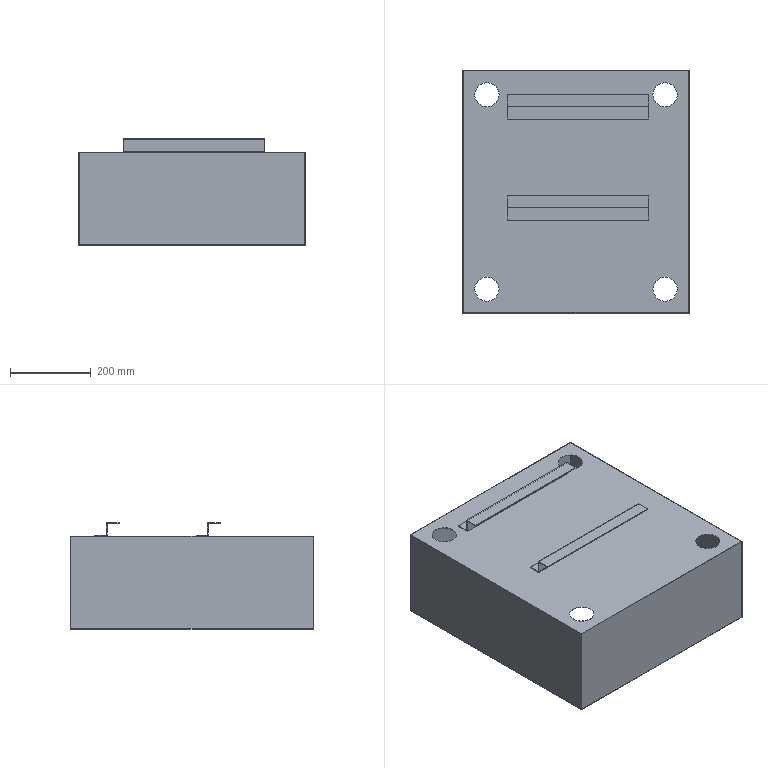Part | SolidWorks | features BaseBody 1 | 1 solid | 47 faces | box 560 x 600 x 263 mm | volume 1044894 mm3 | plane 39 | cylinder 8 | commonest cylinder face diameters 60 x8
STEP:
#1=CARTESIAN_POINT('',(530.,540.,230.));
#2=VERTEX_POINT('',#1);
#3=CARTESIAN_POINT('',(470.,540.,230.));
#4=VERTEX_POINT('',#3);
#5=CARTESIAN_POINT('',(500.,540.,230.));
#6=DIRECTION('',(0.,0.,-1.));
#7=DIRECTION('',(-1.,0.,0.));
#8=AXIS2_PLACEMENT_3D('',#5,#6,#7);
#9=CIRCLE('',#8,30.);
#10=EDGE_CURVE('',#2,#4,#9,.T.);
#11=ORIENTED_EDGE('',*,*,#10,.F.);
#12=CARTESIAN_POINT('',(530.,540.,229.));
#13=VERTEX_POINT('',#12);
#14=CARTESIAN_POINT('',(530.,540.,263.));
#15=DIRECTION('',(0.,0.,-1.));
#16=VECTOR('',#15,1000.);
#17=LINE('',#14,#16);
#18=EDGE_CURVE('',#2,#13,#17,.T.);
#19=ORIENTED_EDGE('',*,*,#18,.T.);
#20=CARTESIAN_POINT('',(470.,540.,229.));
#21=VERTEX_POINT('',#20);
#22=CARTESIAN_POINT('',(500.,540.,229.));
#23=DIRECTION('',(0.,0.,1.));
#24=DIRECTION('',(-1.,0.,0.));
#25=AXIS2_PLACEMENT_3D('',#22,#23,#24);
#26=CIRCLE('',#25,30.);
#27=EDGE_CURVE('',#21,#13,#26,.T.);
#28=ORIENTED_EDGE('',*,*,#27,.F.);
#29=CARTESIAN_POINT('',(470.,540.,263.));
#30=DIRECTION('',(0.,0.,-1.));
#31=VECTOR('',#30,1000.);
#32=LINE('',#29,#31);
#33=EDGE_CURVE('',#4,#21,#32,.T.);
#34=ORIENTED_EDGE('',*,*,#33,.F.);
#35=EDGE_LOOP('',(#11,#19,#28,#34));
#36=FACE_OUTER_BOUND('',#35,.T.);
#37=CARTESIAN_POINT('',(500.,540.,263.));
#38=DIRECTION('',(0.,0.,-1.));
#39=DIRECTION('',(-1.,0.,0.));
#40=AXIS2_PLACEMENT_3D('',#37,#38,#39);
#41=CYLINDRICAL_SURFACE('',#40,30.);
#42=ADVANCED_FACE('',(#36),#41,.F.);
#43=CARTESIAN_POINT('',(90.,540.,230.));
#44=VERTEX_POINT('',#43);
#45=CARTESIAN_POINT('',(30.,540.,230.));
#46=VERTEX_POINT('',#45);
#47=CARTESIAN_POINT('',(60.,540.,230.));
#48=DIRECTION('',(0.,0.,-1.));
#49=DIRECTION('',(-1.,0.,0.));
#50=AXIS2_PLACEMENT_3D('',#47,#48,#49);
#51=CIRCLE('',#50,30.);
#52=EDGE_CURVE('',#44,#46,#51,.T.);
#53=ORIENTED_EDGE('',*,*,#52,.F.);
#54=CARTESIAN_POINT('',(90.,540.,229.));
#55=VERTEX_POINT('',#54);
#56=CARTESIAN_POINT('',(90.,540.,263.));
#57=DIRECTION('',(0.,0.,-1.));
#58=VECTOR('',#57,1000.);
#59=LINE('',#56,#58);
#60=EDGE_CURVE('',#44,#55,#59,.T.);
#61=ORIENTED_EDGE('',*,*,#60,.T.);
#62=CARTESIAN_POINT('',(30.,540.,229.));
#63=VERTEX_POINT('',#62);
#64=CARTESIAN_POINT('',(60.,540.,229.));
#65=DIRECTION('',(0.,0.,1.));
#66=DIRECTION('',(-1.,0.,0.));
#67=AXIS2_PLACEMENT_3D('',#64,#65,#66);
#68=CIRCLE('',#67,30.);
#69=EDGE_CURVE('',#63,#55,#68,.T.);
#70=ORIENTED_EDGE('',*,*,#69,.F.);
#71=CARTESIAN_POINT('',(30.,540.,263.));
#72=DIRECTION('',(0.,0.,-1.));
#73=VECTOR('',#72,1000.);
#74=LINE('',#71,#73);
#75=EDGE_CURVE('',#46,#63,#74,.T.);
#76=ORIENTED_EDGE('',*,*,#75,.F.);
#77=EDGE_LOOP('',(#53,#61,#70,#76));
#78=FACE_OUTER_BOUND('',#77,.T.);
#79=CARTESIAN_POINT('',(60.,540.,263.));
#80=DIRECTION('',(0.,0.,-1.));
#81=DIRECTION('',(-1.,0.,0.));
#82=AXIS2_PLACEMENT_3D('',#79,#80,#81);
#83=CYLINDRICAL_SURFACE('',#82,30.);
#84=ADVANCED_FACE('',(#78),#83,.F.);
#85=CARTESIAN_POINT('',(90.,60.,230.));
#86=VERTEX_POINT('',#85);
#87=CARTESIAN_POINT('',(30.,60.,230.));
#88=VERTEX_POINT('',#87);
#89=CARTESIAN_POINT('',(60.,60.,230.));
#90=DIRECTION('',(0.,0.,-1.));
#91=DIRECTION('',(-1.,0.,0.));
#92=AXIS2_PLACEMENT_3D('',#89,#90,#91);
#93=CIRCLE('',#92,30.);
#94=EDGE_CURVE('',#86,#88,#93,.T.);
#95=ORIENTED_EDGE('',*,*,#94,.F.);
#96=CARTESIAN_POINT('',(90.,60.,229.));
#97=VERTEX_POINT('',#96);
#98=CARTESIAN_POINT('',(90.,60.,263.));
#99=DIRECTION('',(0.,0.,-1.));
#100=VECTOR('',#99,1000.);
#101=LINE('',#98,#100);
#102=EDGE_CURVE('',#86,#97,#101,.T.);
#103=ORIENTED_EDGE('',*,*,#102,.T.);
#104=CARTESIAN_POINT('',(30.,60.,229.));
#105=VERTEX_POINT('',#104);
#106=CARTESIAN_POINT('',(60.,60.,229.));
#107=DIRECTION('',(0.,0.,1.));
#108=DIRECTION('',(-1.,0.,0.));
#109=AXIS2_PLACEMENT_3D('',#106,#107,#108);
#110=CIRCLE('',#109,30.);
#111=EDGE_CURVE('',#105,#97,#110,.T.);
#112=ORIENTED_EDGE('',*,*,#111,.F.);
#113=CARTESIAN_POINT('',(30.,60.,263.));
#114=DIRECTION('',(0.,0.,-1.));
#115=VECTOR('',#114,1000.);
#116=LINE('',#113,#115);
#117=EDGE_CURVE('',#88,#105,#116,.T.);
#118=ORIENTED_EDGE('',*,*,#117,.F.);
#119=EDGE_LOOP('',(#95,#103,#112,#118));
#120=FACE_OUTER_BOUND('',#119,.T.);
#121=CARTESIAN_POINT('',(60.,60.,263.));
#122=DIRECTION('',(0.,0.,-1.));
#123=DIRECTION('',(-1.,0.,0.));
#124=AXIS2_PLACEMENT_3D('',#121,#122,#123);
#125=CYLINDRICAL_SURFACE('',#124,30.);
#126=ADVANCED_FACE('',(#120),#125,.F.);
#127=CARTESIAN_POINT('',(530.,60.,230.));
#128=VERTEX_POINT('',#127);
#129=CARTESIAN_POINT('',(470.,60.,230.));
#130=VERTEX_POINT('',#129);
#131=CARTESIAN_POINT('',(500.,60.,230.));
#132=DIRECTION('',(0.,0.,-1.));
#133=DIRECTION('',(-1.,0.,0.));
#134=AXIS2_PLACEMENT_3D('',#131,#132,#133);
#135=CIRCLE('',#134,30.);
#136=EDGE_CURVE('',#128,#130,#135,.T.);
#137=ORIENTED_EDGE('',*,*,#136,.F.);
#138=CARTESIAN_POINT('',(530.,60.,229.));
#139=VERTEX_POINT('',#138);
#140=CARTESIAN_POINT('',(530.,60.,263.));
#141=DIRECTION('',(0.,0.,-1.));
#142=VECTOR('',#141,1000.);
#143=LINE('',#140,#142);
#144=EDGE_CURVE('',#128,#139,#143,.T.);
#145=ORIENTED_EDGE('',*,*,#144,.T.);
#146=CARTESIAN_POINT('',(470.,60.,229.));
#147=VERTEX_POINT('',#146);
#148=CARTESIAN_POINT('',(500.,60.,229.));
#149=DIRECTION('',(0.,0.,1.));
#150=DIRECTION('',(-1.,0.,0.));
#151=AXIS2_PLACEMENT_3D('',#148,#149,#150);
#152=CIRCLE('',#151,30.);
#153=EDGE_CURVE('',#147,#139,#152,.T.);
#154=ORIENTED_EDGE('',*,*,#153,.F.);
#155=CARTESIAN_POINT('',(470.,60.,263.));
#156=DIRECTION('',(0.,0.,-1.));
#157=VECTOR('',#156,1000.);
#158=LINE('',#155,#157);
#159=EDGE_CURVE('',#130,#147,#158,.T.);
#160=ORIENTED_EDGE('',*,*,#159,.F.);
#161=EDGE_LOOP('',(#137,#145,#154,#160));
#162=FACE_OUTER_BOUND('',#161,.T.);
#163=CARTESIAN_POINT('',(500.,60.,263.));
#164=DIRECTION('',(0.,0.,-1.));
#165=DIRECTION('',(-1.,0.,0.));
#166=AXIS2_PLACEMENT_3D('',#163,#164,#165);
#167=CYLINDRICAL_SURFACE('',#166,30.);
#168=ADVANCED_FACE('',(#162),#167,.F.);
#169=CARTESIAN_POINT('',(559.,599.,229.));
#170=VERTEX_POINT('',#169);
#171=CARTESIAN_POINT('',(559.,1.,229.));
#172=VERTEX_POINT('',#171);
#173=CARTESIAN_POINT('',(559.,0.,229.));
#174=DIRECTION('',(0.,-1.,0.));
#175=VECTOR('',#174,1000.);
#176=LINE('',#173,#175);
#177=EDGE_CURVE('',#170,#172,#176,.T.);
#178=ORIENTED_EDGE('',*,*,#177,.T.);
#179=CARTESIAN_POINT('',(1.,1.,229.));
#180=VERTEX_POINT('',#179);
#181=CARTESIAN_POINT('',(0.,1.,229.));
#182=DIRECTION('',(-1.,0.,0.));
#183=VECTOR('',#182,1000.);
#184=LINE('',#181,#183);
#185=EDGE_CURVE('',#172,#180,#184,.T.);
#186=ORIENTED_EDGE('',*,*,#185,.T.);
#187=CARTESIAN_POINT('',(1.,599.,229.));
#188=VERTEX_POINT('',#187);
#189=CARTESIAN_POINT('',(1.,0.,229.));
#190=DIRECTION('',(0.,1.,0.));
#191=VECTOR('',#190,1000.);
#192=LINE('',#189,#191);
#193=EDGE_CURVE('',#180,#188,#192,.T.);
#194=ORIENTED_EDGE('',*,*,#193,.T.);
#195=CARTESIAN_POINT('',(0.,599.,229.));
#196=DIRECTION('',(1.,0.,0.));
#197=VECTOR('',#196,1000.);
#198=LINE('',#195,#197);
#199=EDGE_CURVE('',#188,#170,#198,.T.);
#200=ORIENTED_EDGE('',*,*,#199,.T.);
#201=EDGE_LOOP('',(#178,#186,#194,#200));
#202=FACE_OUTER_BOUND('',#201,.T.);
#203=ORIENTED_EDGE('',*,*,#27,.T.);
#204=CARTESIAN_POINT('',(500.,540.,229.));
#205=DIRECTION('',(0.,0.,1.));
#206=DIRECTION('',(-1.,0.,0.));
#207=AXIS2_PLACEMENT_3D('',#204,#205,#206);
#208=CIRCLE('',#207,30.);
#209=EDGE_CURVE('',#13,#21,#208,.T.);
#210=ORIENTED_EDGE('',*,*,#209,.T.);
#211=EDGE_LOOP('',(#203,#210));
#212=FACE_BOUND('',#211,.T.);
#213=ORIENTED_EDGE('',*,*,#69,.T.);
#214=CARTESIAN_POINT('',(60.,540.,229.));
#215=DIRECTION('',(0.,0.,1.));
#216=DIRECTION('',(-1.,0.,0.));
#217=AXIS2_PLACEMENT_3D('',#214,#215,#216);
#218=CIRCLE('',#217,30.);
#219=EDGE_CURVE('',#55,#63,#218,.T.);
#220=ORIENTED_EDGE('',*,*,#219,.T.);
#221=EDGE_LOOP('',(#213,#220));
#222=FACE_BOUND('',#221,.T.);
#223=ORIENTED_EDGE('',*,*,#111,.T.);
#224=CARTESIAN_POINT('',(60.,60.,229.));
#225=DIRECTION('',(0.,0.,1.));
#226=DIRECTION('',(-1.,0.,0.));
#227=AXIS2_PLACEMENT_3D('',#224,#225,#226);
#228=CIRCLE('',#227,30.);
#229=EDGE_CURVE('',#97,#105,#228,.T.);
#230=ORIENTED_EDGE('',*,*,#229,.T.);
#231=EDGE_LOOP('',(#223,#230));
#232=FACE_BOUND('',#231,.T.);
#233=ORIENTED_EDGE('',*,*,#153,.T.);
#234=CARTESIAN_POINT('',(500.,60.,229.));
#235=DIRECTION('',(0.,0.,1.));
#236=DIRECTION('',(-1.,0.,0.));
#237=AXIS2_PLACEMENT_3D('',#234,#235,#236);
#238=CIRCLE('',#237,30.);
#239=EDGE_CURVE('',#139,#147,#238,.T.);
#240=ORIENTED_EDGE('',*,*,#239,.T.);
#241=EDGE_LOOP('',(#233,#240));
#242=FACE_BOUND('',#241,.T.);
#243=CARTESIAN_POINT('',(0.,0.,229.));
#244=DIRECTION('',(0.,0.,-1.));
#245=DIRECTION('',(-1.,0.,0.));
#246=AXIS2_PLACEMENT_3D('',#243,#244,#245);
#247=PLANE('',#246);
#248=ADVANCED_FACE('',(#202,#212,#222,#232,#242),#247,.T.);
#249=ORIENTED_EDGE('',*,*,#185,.F.);
#250=CARTESIAN_POINT('',(559.,1.,1.));
#251=VERTEX_POINT('',#250);
#252=CARTESIAN_POINT('',(559.,1.,230.));
#253=DIRECTION('',(0.,0.,-1.));
#254=VECTOR('',#253,1000.);
#255=LINE('',#252,#254);
#256=EDGE_CURVE('',#172,#251,#255,.T.);
#257=ORIENTED_EDGE('',*,*,#256,.T.);
#258=CARTESIAN_POINT('',(1.,1.,1.));
#259=VERTEX_POINT('',#258);
#260=CARTESIAN_POINT('',(0.,1.,1.));
#261=DIRECTION('',(-1.,0.,0.));
#262=VECTOR('',#261,1000.);
#263=LINE('',#260,#262);
#264=EDGE_CURVE('',#251,#259,#263,.T.);
#265=ORIENTED_EDGE('',*,*,#264,.T.);
#266=CARTESIAN_POINT('',(1.,1.,230.));
#267=DIRECTION('',(0.,0.,1.));
#268=VECTOR('',#267,1000.);
#269=LINE('',#266,#268);
#270=EDGE_CURVE('',#259,#180,#269,.T.);
#271=ORIENTED_EDGE('',*,*,#270,.T.);
#272=EDGE_LOOP('',(#249,#257,#265,#271));
#273=FACE_OUTER_BOUND('',#272,.T.);
#274=CARTESIAN_POINT('',(0.,1.,230.));
#275=DIRECTION('',(0.,1.,0.));
#276=DIRECTION('',(0.,0.,1.));
#277=AXIS2_PLACEMENT_3D('',#274,#275,#276);
#278=PLANE('',#277);
#279=ADVANCED_FACE('',(#273),#278,.T.);
#280=ORIENTED_EDGE('',*,*,#177,.F.);
#281=CARTESIAN_POINT('',(559.,599.,1.));
#282=VERTEX_POINT('',#281);
#283=CARTESIAN_POINT('',(559.,599.,230.));
#284=DIRECTION('',(0.,0.,-1.));
#285=VECTOR('',#284,1000.);
#286=LINE('',#283,#285);
#287=EDGE_CURVE('',#170,#282,#286,.T.);
#288=ORIENTED_EDGE('',*,*,#287,.T.);
#289=CARTESIAN_POINT('',(559.,0.,1.));
#290=DIRECTION('',(0.,-1.,0.));
#291=VECTOR('',#290,1000.);
#292=LINE('',#289,#291);
#293=EDGE_CURVE('',#282,#251,#292,.T.);
#294=ORIENTED_EDGE('',*,*,#293,.T.);
#295=ORIENTED_EDGE('',*,*,#256,.F.);
#296=EDGE_LOOP('',(#280,#288,#294,#295));
#297=FACE_OUTER_BOUND('',#296,.T.);
#298=CARTESIAN_POINT('',(559.,0.,230.));
#299=DIRECTION('',(-1.,0.,0.));
#300=DIRECTION('',(0.,0.,1.));
#301=AXIS2_PLACEMENT_3D('',#298,#299,#300);
#302=PLANE('',#301);
#303=ADVANCED_FACE('',(#297),#302,.T.);
#304=ORIENTED_EDGE('',*,*,#199,.F.);
#305=CARTESIAN_POINT('',(1.,599.,1.));
#306=VERTEX_POINT('',#305);
#307=CARTESIAN_POINT('',(1.,599.,230.));
#308=DIRECTION('',(0.,0.,-1.));
#309=VECTOR('',#308,1000.);
#310=LINE('',#307,#309);
#311=EDGE_CURVE('',#188,#306,#310,.T.);
#312=ORIENTED_EDGE('',*,*,#311,.T.);
#313=CARTESIAN_POINT('',(0.,599.,1.));
#314=DIRECTION('',(1.,0.,0.));
#315=VECTOR('',#314,1000.);
#316=LINE('',#313,#315);
#317=EDGE_CURVE('',#306,#282,#316,.T.);
#318=ORIENTED_EDGE('',*,*,#317,.T.);
#319=ORIENTED_EDGE('',*,*,#287,.F.);
#320=EDGE_LOOP('',(#304,#312,#318,#319));
#321=FACE_OUTER_BOUND('',#320,.T.);
#322=CARTESIAN_POINT('',(0.,599.,230.));
#323=DIRECTION('',(0.,-1.,0.));
#324=DIRECTION('',(0.,0.,-1.));
#325=AXIS2_PLACEMENT_3D('',#322,#323,#324);
#326=PLANE('',#325);
#327=ADVANCED_FACE('',(#321),#326,.T.);
#328=ORIENTED_EDGE('',*,*,#193,.F.);
#329=ORIENTED_EDGE('',*,*,#270,.F.);
#330=CARTESIAN_POINT('',(1.,0.,1.));
#331=DIRECTION('',(0.,1.,0.));
#332=VECTOR('',#331,1000.);
#333=LINE('',#330,#332);
#334=EDGE_CURVE('',#259,#306,#333,.T.);
#335=ORIENTED_EDGE('',*,*,#334,.T.);
#336=ORIENTED_EDGE('',*,*,#311,.F.);
#337=EDGE_LOOP('',(#328,#329,#335,#336));
#338=FACE_OUTER_BOUND('',#337,.T.);
#339=CARTESIAN_POINT('',(1.,0.,230.));
#340=DIRECTION('',(1.,0.,0.));
#341=DIRECTION('',(0.,0.,-1.));
#342=AXIS2_PLACEMENT_3D('',#339,#340,#341);
#343=PLANE('',#342);
#344=ADVANCED_FACE('',(#338),#343,.T.);
#345=ORIENTED_EDGE('',*,*,#18,.F.);
#346=CARTESIAN_POINT('',(500.,540.,230.));
#347=DIRECTION('',(0.,0.,-1.));
#348=DIRECTION('',(-1.,0.,0.));
#349=AXIS2_PLACEMENT_3D('',#346,#347,#348);
#350=CIRCLE('',#349,30.);
#351=EDGE_CURVE('',#4,#2,#350,.T.);
#352=ORIENTED_EDGE('',*,*,#351,.F.);
#353=ORIENTED_EDGE('',*,*,#33,.T.);
#354=ORIENTED_EDGE('',*,*,#209,.F.);
#355=EDGE_LOOP('',(#345,#352,#353,#354));
#356=FACE_OUTER_BOUND('',#355,.T.);
#357=CARTESIAN_POINT('',(500.,540.,263.));
#358=DIRECTION('',(0.,0.,-1.));
#359=DIRECTION('',(-1.,0.,0.));
#360=AXIS2_PLACEMENT_3D('',#357,#358,#359);
#361=CYLINDRICAL_SURFACE('',#360,30.);
#362=ADVANCED_FACE('',(#356),#361,.F.);
#363=ORIENTED_EDGE('',*,*,#60,.F.);
#364=CARTESIAN_POINT('',(60.,540.,230.));
#365=DIRECTION('',(0.,0.,-1.));
#366=DIRECTION('',(-1.,0.,0.));
#367=AXIS2_PLACEMENT_3D('',#364,#365,#366);
#368=CIRCLE('',#367,30.);
#369=EDGE_CURVE('',#46,#44,#368,.T.);
#370=ORIENTED_EDGE('',*,*,#369,.F.);
#371=ORIENTED_EDGE('',*,*,#75,.T.);
#372=ORIENTED_EDGE('',*,*,#219,.F.);
#373=EDGE_LOOP('',(#363,#370,#371,#372));
#374=FACE_OUTER_BOUND('',#373,.T.);
#375=CARTESIAN_POINT('',(60.,540.,263.));
#376=DIRECTION('',(0.,0.,-1.));
#377=DIRECTION('',(-1.,0.,0.));
#378=AXIS2_PLACEMENT_3D('',#375,#376,#377);
#379=CYLINDRICAL_SURFACE('',#378,30.);
#380=ADVANCED_FACE('',(#374),#379,.F.);
#381=ORIENTED_EDGE('',*,*,#102,.F.);
#382=CARTESIAN_POINT('',(60.,60.,230.));
#383=DIRECTION('',(0.,0.,-1.));
#384=DIRECTION('',(-1.,0.,0.));
#385=AXIS2_PLACEMENT_3D('',#382,#383,#384);
#386=CIRCLE('',#385,30.);
#387=EDGE_CURVE('',#88,#86,#386,.T.);
#388=ORIENTED_EDGE('',*,*,#387,.F.);
#389=ORIENTED_EDGE('',*,*,#117,.T.);
#390=ORIENTED_EDGE('',*,*,#229,.F.);
#391=EDGE_LOOP('',(#381,#388,#389,#390));
#392=FACE_OUTER_BOUND('',#391,.T.);
#393=CARTESIAN_POINT('',(60.,60.,263.));
#394=DIRECTION('',(0.,0.,-1.));
#395=DIRECTION('',(-1.,0.,0.));
#396=AXIS2_PLACEMENT_3D('',#393,#394,#395);
#397=CYLINDRICAL_SURFACE('',#396,30.);
#398=ADVANCED_FACE('',(#392),#397,.F.);
#399=ORIENTED_EDGE('',*,*,#144,.F.);
#400=CARTESIAN_POINT('',(500.,60.,230.));
#401=DIRECTION('',(0.,0.,-1.));
#402=DIRECTION('',(-1.,0.,0.));
#403=AXIS2_PLACEMENT_3D('',#400,#401,#402);
#404=CIRCLE('',#403,30.);
#405=EDGE_CURVE('',#130,#128,#404,.T.);
#406=ORIENTED_EDGE('',*,*,#405,.F.);
#407=ORIENTED_EDGE('',*,*,#159,.T.);
#408=ORIENTED_EDGE('',*,*,#239,.F.);
#409=EDGE_LOOP('',(#399,#406,#407,#408));
#410=FACE_OUTER_BOUND('',#409,.T.);
#411=CARTESIAN_POINT('',(500.,60.,263.));
#412=DIRECTION('',(0.,0.,-1.));
#413=DIRECTION('',(-1.,0.,0.));
#414=AXIS2_PLACEMENT_3D('',#411,#412,#413);
#415=CYLINDRICAL_SURFACE('',#414,30.);
#416=ADVANCED_FACE('',(#410),#415,.F.);
#417=ORIENTED_EDGE('',*,*,#264,.F.);
#418=ORIENTED_EDGE('',*,*,#293,.F.);
#419=ORIENTED_EDGE('',*,*,#317,.F.);
#420=ORIENTED_EDGE('',*,*,#334,.F.);
#421=EDGE_LOOP('',(#417,#418,#419,#420));
#422=FACE_OUTER_BOUND('',#421,.T.);
#423=CARTESIAN_POINT('',(14.,14.,1.));
#424=VERTEX_POINT('',#423);
#425=CARTESIAN_POINT('',(546.,14.,1.));
#426=VERTEX_POINT('',#425);
#427=CARTESIAN_POINT('',(0.,14.,1.));
#428=DIRECTION('',(1.,0.,0.));
#429=VECTOR('',#428,1000.);
#430=LINE('',#427,#429);
#431=EDGE_CURVE('',#424,#426,#430,.T.);
#432=ORIENTED_EDGE('',*,*,#431,.F.);
#433=CARTESIAN_POINT('',(14.,586.,1.));
#434=VERTEX_POINT('',#433);
#435=CARTESIAN_POINT('',(14.,0.,1.));
#436=DIRECTION('',(0.,-1.,0.));
#437=VECTOR('',#436,1000.);
#438=LINE('',#435,#437);
#439=EDGE_CURVE('',#434,#424,#438,.T.);
#440=ORIENTED_EDGE('',*,*,#439,.F.);
#441=CARTESIAN_POINT('',(546.,586.,1.));
#442=VERTEX_POINT('',#441);
#443=CARTESIAN_POINT('',(0.,586.,1.));
#444=DIRECTION('',(-1.,0.,0.));
#445=VECTOR('',#444,1000.);
#446=LINE('',#443,#445);
#447=EDGE_CURVE('',#442,#434,#446,.T.);
#448=ORIENTED_EDGE('',*,*,#447,.F.);
#449=CARTESIAN_POINT('',(546.,0.,1.));
#450=DIRECTION('',(0.,1.,0.));
#451=VECTOR('',#450,1000.);
#452=LINE('',#449,#451);
#453=EDGE_CURVE('',#426,#442,#452,.T.);
#454=ORIENTED_EDGE('',*,*,#453,.F.);
#455=EDGE_LOOP('',(#432,#440,#448,#454));
#456=FACE_BOUND('',#455,.T.);
#457=CARTESIAN_POINT('',(0.,0.,1.));
#458=DIRECTION('',(0.,0.,-1.));
#459=DIRECTION('',(-1.,0.,0.));
#460=AXIS2_PLACEMENT_3D('',#457,#458,#459);
#461=PLANE('',#460);
#462=ADVANCED_FACE('',(#422,#456),#461,.F.);
#463=CARTESIAN_POINT('',(460.,290.,230.));
#464=VERTEX_POINT('',#463);
#465=CARTESIAN_POINT('',(110.,290.,230.));
#466=VERTEX_POINT('',#465);
#467=CARTESIAN_POINT('',(0.,290.,230.));
#468=DIRECTION('',(-1.,0.,0.));
#469=VECTOR('',#468,1000.);
#470=LINE('',#467,#469);
#471=EDGE_CURVE('',#464,#466,#470,.T.);
#472=ORIENTED_EDGE('',*,*,#471,.F.);
#473=CARTESIAN_POINT('',(460.,260.,230.));
#474=VERTEX_POINT('',#473);
#475=CARTESIAN_POINT('',(460.,0.,230.));
#476=DIRECTION('',(0.,1.,0.));
#477=VECTOR('',#476,1000.);
#478=LINE('',#475,#477);
#479=EDGE_CURVE('',#474,#464,#478,.T.);
#480=ORIENTED_EDGE('',*,*,#479,.F.);
#481=CARTESIAN_POINT('',(110.,260.,230.));
#482=VERTEX_POINT('',#481);
#483=CARTESIAN_POINT('',(0.,260.,230.));
#484=DIRECTION('',(1.,0.,0.));
#485=VECTOR('',#484,1000.);
#486=LINE('',#483,#485);
#487=EDGE_CURVE('',#482,#474,#486,.T.);
#488=ORIENTED_EDGE('',*,*,#487,.F.);
#489=CARTESIAN_POINT('',(110.,0.,230.));
#490=DIRECTION('',(0.,-1.,0.));
#491=VECTOR('',#490,1000.);
#492=LINE('',#489,#491);
#493=EDGE_CURVE('',#466,#482,#492,.T.);
#494=ORIENTED_EDGE('',*,*,#493,.F.);
#495=EDGE_LOOP('',(#472,#480,#488,#494));
#496=FACE_BOUND('',#495,.T.);
#497=CARTESIAN_POINT('',(560.,0.,230.));
#498=VERTEX_POINT('',#497);
#499=CARTESIAN_POINT('',(0.,0.,230.));
#500=VERTEX_POINT('',#499);
#501=CARTESIAN_POINT('',(0.,0.,230.));
#502=DIRECTION('',(-1.,0.,0.));
#503=VECTOR('',#502,1000.);
#504=LINE('',#501,#503);
#505=EDGE_CURVE('',#498,#500,#504,.T.);
#506=ORIENTED_EDGE('',*,*,#505,.F.);
#507=CARTESIAN_POINT('',(560.,600.,230.));
#508=VERTEX_POINT('',#507);
#509=CARTESIAN_POINT('',(560.,0.,230.));
#510=DIRECTION('',(0.,-1.,0.));
#511=VECTOR('',#510,1000.);
#512=LINE('',#509,#511);
#513=EDGE_CURVE('',#508,#498,#512,.T.);
#514=ORIENTED_EDGE('',*,*,#513,.F.);
#515=CARTESIAN_POINT('',(0.,600.,230.));
#516=VERTEX_POINT('',#515);
#517=CARTESIAN_POINT('',(0.,600.,230.));
#518=DIRECTION('',(1.,0.,0.));
#519=VECTOR('',#518,1000.);
#520=LINE('',#517,#519);
#521=EDGE_CURVE('',#516,#508,#520,.T.);
#522=ORIENTED_EDGE('',*,*,#521,.F.);
#523=CARTESIAN_POINT('',(0.,0.,230.));
#524=DIRECTION('',(0.,1.,0.));
#525=VECTOR('',#524,1000.);
#526=LINE('',#523,#525);
#527=EDGE_CURVE('',#500,#516,#526,.T.);
#528=ORIENTED_EDGE('',*,*,#527,.F.);
#529=EDGE_LOOP('',(#506,#514,#522,#528));
#530=FACE_OUTER_BOUND('',#529,.T.);
#531=CARTESIAN_POINT('',(110.,540.,230.));
#532=VERTEX_POINT('',#531);
#533=CARTESIAN_POINT('',(110.,510.,230.));
#534=VERTEX_POINT('',#533);
#535=CARTESIAN_POINT('',(110.,0.,230.));
#536=DIRECTION('',(0.,-1.,0.));
#537=VECTOR('',#536,1000.);
#538=LINE('',#535,#537);
#539=EDGE_CURVE('',#532,#534,#538,.T.);
#540=ORIENTED_EDGE('',*,*,#539,.F.);
#541=CARTESIAN_POINT('',(460.,540.,230.));
#542=VERTEX_POINT('',#541);
#543=CARTESIAN_POINT('',(0.,540.,230.));
#544=DIRECTION('',(-1.,0.,0.));
#545=VECTOR('',#544,1000.);
#546=LINE('',#543,#545);
#547=EDGE_CURVE('',#542,#532,#546,.T.);
#548=ORIENTED_EDGE('',*,*,#547,.F.);
#549=CARTESIAN_POINT('',(460.,510.,230.));
#550=VERTEX_POINT('',#549);
#551=CARTESIAN_POINT('',(460.,0.,230.));
#552=DIRECTION('',(0.,1.,0.));
#553=VECTOR('',#552,1000.);
#554=LINE('',#551,#553);
#555=EDGE_CURVE('',#550,#542,#554,.T.);
#556=ORIENTED_EDGE('',*,*,#555,.F.);
#557=CARTESIAN_POINT('',(0.,510.,230.));
#558=DIRECTION('',(1.,0.,0.));
#559=VECTOR('',#558,1000.);
#560=LINE('',#557,#559);
#561=EDGE_CURVE('',#534,#550,#560,.T.);
#562=ORIENTED_EDGE('',*,*,#561,.F.);
#563=EDGE_LOOP('',(#540,#548,#556,#562));
#564=FACE_BOUND('',#563,.T.);
#565=ORIENTED_EDGE('',*,*,#351,.T.);
#566=ORIENTED_EDGE('',*,*,#10,.T.);
#567=EDGE_LOOP('',(#565,#566));
#568=FACE_BOUND('',#567,.T.);
#569=ORIENTED_EDGE('',*,*,#369,.T.);
#570=ORIENTED_EDGE('',*,*,#52,.T.);
#571=EDGE_LOOP('',(#569,#570));
#572=FACE_BOUND('',#571,.T.);
#573=ORIENTED_EDGE('',*,*,#387,.T.);
#574=ORIENTED_EDGE('',*,*,#94,.T.);
#575=EDGE_LOOP('',(#573,#574));
#576=FACE_BOUND('',#575,.T.);
#577=ORIENTED_EDGE('',*,*,#405,.T.);
#578=ORIENTED_EDGE('',*,*,#136,.T.);
#579=EDGE_LOOP('',(#577,#578));
#580=FACE_BOUND('',#579,.T.);
#581=CARTESIAN_POINT('',(0.,0.,230.));
#582=DIRECTION('',(0.,0.,-1.));
#583=DIRECTION('',(-1.,0.,0.));
#584=AXIS2_PLACEMENT_3D('',#581,#582,#583);
#585=PLANE('',#584);
#586=ADVANCED_FACE('',(#496,#530,#564,#568,#572,#576,#580),#585,.F.);
#587=CARTESIAN_POINT('',(546.,586.,15.));
#588=VERTEX_POINT('',#587);
#589=CARTESIAN_POINT('',(546.,14.,15.));
#590=VERTEX_POINT('',#589);
#591=CARTESIAN_POINT('',(546.,585.,15.));
#592=DIRECTION('',(0.,-1.,0.));
#593=VECTOR('',#592,1000.);
#594=LINE('',#591,#593);
#595=EDGE_CURVE('',#588,#590,#594,.T.);
#596=ORIENTED_EDGE('',*,*,#595,.T.);
#597=CARTESIAN_POINT('',(546.,14.,15.));
#598=DIRECTION('',(0.,0.,-1.));
#599=VECTOR('',#598,1000.);
#600=LINE('',#597,#599);
#601=EDGE_CURVE('',#590,#426,#600,.T.);
#602=ORIENTED_EDGE('',*,*,#601,.T.);
#603=ORIENTED_EDGE('',*,*,#453,.T.);
#604=CARTESIAN_POINT('',(546.,586.,15.));
#605=DIRECTION('',(0.,0.,1.));
#606=VECTOR('',#605,1000.);
#607=LINE('',#604,#606);
#608=EDGE_CURVE('',#442,#588,#607,.T.);
#609=ORIENTED_EDGE('',*,*,#608,.T.);
#610=EDGE_LOOP('',(#596,#602,#603,#609));
#611=FACE_OUTER_BOUND('',#610,.T.);
#612=CARTESIAN_POINT('',(546.,585.,15.));
#613=DIRECTION('',(1.,0.,0.));
#614=DIRECTION('',(0.,1.,0.));
#615=AXIS2_PLACEMENT_3D('',#612,#613,#614);
#616=PLANE('',#615);
#617=ADVANCED_FACE('',(#611),#616,.T.);
#618=CARTESIAN_POINT('',(14.,14.,15.));
#619=VERTEX_POINT('',#618);
#620=CARTESIAN_POINT('',(545.,14.,15.));
#621=DIRECTION('',(-1.,0.,0.));
#622=VECTOR('',#621,1000.);
#623=LINE('',#620,#622);
#624=EDGE_CURVE('',#590,#619,#623,.T.);
#625=ORIENTED_EDGE('',*,*,#624,.T.);
#626=CARTESIAN_POINT('',(14.,14.,15.));
#627=DIRECTION('',(0.,0.,-1.));
#628=VECTOR('',#627,1000.);
#629=LINE('',#626,#628);
#630=EDGE_CURVE('',#619,#424,#629,.T.);
#631=ORIENTED_EDGE('',*,*,#630,.T.);
#632=ORIENTED_EDGE('',*,*,#431,.T.);
#633=ORIENTED_EDGE('',*,*,#601,.F.);
#634=EDGE_LOOP('',(#625,#631,#632,#633));
#635=FACE_OUTER_BOUND('',#634,.T.);
#636=CARTESIAN_POINT('',(545.,14.,15.));
#637=DIRECTION('',(0.,-1.,0.));
#638=DIRECTION('',(0.,0.,-1.));
#639=AXIS2_PLACEMENT_3D('',#636,#637,#638);
#640=PLANE('',#639);
#641=ADVANCED_FACE('',(#635),#640,.T.);
#642=CARTESIAN_POINT('',(14.,586.,15.));
#643=VERTEX_POINT('',#642);
#644=CARTESIAN_POINT('',(14.,585.,15.));
#645=DIRECTION('',(0.,1.,0.));
#646=VECTOR('',#645,1000.);
#647=LINE('',#644,#646);
#648=EDGE_CURVE('',#619,#643,#647,.T.);
#649=ORIENTED_EDGE('',*,*,#648,.T.);
#650=CARTESIAN_POINT('',(14.,586.,15.));
#651=DIRECTION('',(0.,0.,-1.));
#652=VECTOR('',#651,1000.);
#653=LINE('',#650,#652);
#654=EDGE_CURVE('',#643,#434,#653,.T.);
#655=ORIENTED_EDGE('',*,*,#654,.T.);
#656=ORIENTED_EDGE('',*,*,#439,.T.);
#657=ORIENTED_EDGE('',*,*,#630,.F.);
#658=EDGE_LOOP('',(#649,#655,#656,#657));
#659=FACE_OUTER_BOUND('',#658,.T.);
#660=CARTESIAN_POINT('',(14.,585.,15.));
#661=DIRECTION('',(-1.,0.,0.));
#662=DIRECTION('',(0.,-1.,0.));
#663=AXIS2_PLACEMENT_3D('',#660,#661,#662);
#664=PLANE('',#663);
#665=ADVANCED_FACE('',(#659),#664,.T.);
#666=CARTESIAN_POINT('',(545.,586.,15.));
#667=DIRECTION('',(1.,0.,0.));
#668=VECTOR('',#667,1000.);
#669=LINE('',#666,#668);
#670=EDGE_CURVE('',#643,#588,#669,.T.);
#671=ORIENTED_EDGE('',*,*,#670,.T.);
#672=ORIENTED_EDGE('',*,*,#608,.F.);
#673=ORIENTED_EDGE('',*,*,#447,.T.);
#674=ORIENTED_EDGE('',*,*,#654,.F.);
#675=EDGE_LOOP('',(#671,#672,#673,#674));
#676=FACE_OUTER_BOUND('',#675,.T.);
#677=CARTESIAN_POINT('',(545.,586.,15.));
#678=DIRECTION('',(0.,1.,0.));
#679=DIRECTION('',(0.,0.,1.));
#680=AXIS2_PLACEMENT_3D('',#677,#678,#679);
#681=PLANE('',#680);
#682=ADVANCED_FACE('',(#676),#681,.T.);
#683=CARTESIAN_POINT('',(110.,262.,232.));
#684=VERTEX_POINT('',#683);
#685=CARTESIAN_POINT('',(110.,262.,263.));
#686=VERTEX_POINT('',#685);
#687=CARTESIAN_POINT('',(110.,262.,0.));
#688=DIRECTION('',(0.,0.,1.));
#689=VECTOR('',#688,1000.);
#690=LINE('',#687,#689);
#691=EDGE_CURVE('',#684,#686,#690,.T.);
#692=ORIENTED_EDGE('',*,*,#691,.F.);
#693=CARTESIAN_POINT('',(110.,290.,232.));
#694=VERTEX_POINT('',#693);
#695=CARTESIAN_POINT('',(110.,0.,232.));
#696=DIRECTION('',(0.,-1.,0.));
#697=VECTOR('',#696,1000.);
#698=LINE('',#695,#697);
#699=EDGE_CURVE('',#694,#684,#698,.T.);
#700=ORIENTED_EDGE('',*,*,#699,.F.);
#701=CARTESIAN_POINT('',(110.,290.,0.));
#702=DIRECTION('',(0.,0.,1.));
#703=VECTOR('',#702,1000.);
#704=LINE('',#701,#703);
#705=EDGE_CURVE('',#466,#694,#704,.T.);
#706=ORIENTED_EDGE('',*,*,#705,.F.);
#707=ORIENTED_EDGE('',*,*,#493,.T.);
#708=CARTESIAN_POINT('',(110.,260.,261.));
#709=VERTEX_POINT('',#708);
#710=CARTESIAN_POINT('',(110.,260.,0.));
#711=DIRECTION('',(0.,0.,-1.));
#712=VECTOR('',#711,1000.);
#713=LINE('',#710,#712);
#714=EDGE_CURVE('',#709,#482,#713,.T.);
#715=ORIENTED_EDGE('',*,*,#714,.F.);
#716=CARTESIAN_POINT('',(110.,230.,261.));
#717=VERTEX_POINT('',#716);
#718=CARTESIAN_POINT('',(110.,0.,261.));
#719=DIRECTION('',(0.,1.,0.));
#720=VECTOR('',#719,1000.);
#721=LINE('',#718,#720);
#722=EDGE_CURVE('',#717,#709,#721,.T.);
#723=ORIENTED_EDGE('',*,*,#722,.F.);
#724=CARTESIAN_POINT('',(110.,230.,263.));
#725=VERTEX_POINT('',#724);
#726=CARTESIAN_POINT('',(110.,230.,0.));
#727=DIRECTION('',(0.,0.,-1.));
#728=VECTOR('',#727,1000.);
#729=LINE('',#726,#728);
#730=EDGE_CURVE('',#725,#717,#729,.T.);
#731=ORIENTED_EDGE('',*,*,#730,.F.);
#732=CARTESIAN_POINT('',(110.,0.,263.));
#733=DIRECTION('',(0.,-1.,0.));
#734=VECTOR('',#733,1000.);
#735=LINE('',#732,#734);
#736=EDGE_CURVE('',#686,#725,#735,.T.);
#737=ORIENTED_EDGE('',*,*,#736,.F.);
#738=EDGE_LOOP('',(#692,#700,#706,#707,#715,#723,#731,#737));
#739=FACE_OUTER_BOUND('',#738,.T.);
#740=CARTESIAN_POINT('',(110.,0.,0.));
#741=DIRECTION('',(1.,0.,0.));
#742=DIRECTION('',(0.,0.,-1.));
#743=AXIS2_PLACEMENT_3D('',#740,#741,#742);
#744=PLANE('',#743);
#745=ADVANCED_FACE('',(#739),#744,.F.);
#746=ORIENTED_EDGE('',*,*,#471,.T.);
#747=ORIENTED_EDGE('',*,*,#705,.T.);
#748=CARTESIAN_POINT('',(460.,290.,232.));
#749=VERTEX_POINT('',#748);
#750=CARTESIAN_POINT('',(110.,290.,232.));
#751=DIRECTION('',(-1.,0.,0.));
#752=VECTOR('',#751,1000.);
#753=LINE('',#750,#752);
#754=EDGE_CURVE('',#749,#694,#753,.T.);
#755=ORIENTED_EDGE('',*,*,#754,.F.);
#756=CARTESIAN_POINT('',(460.,290.,232.));
#757=DIRECTION('',(0.,0.,1.));
#758=VECTOR('',#757,1000.);
#759=LINE('',#756,#758);
#760=EDGE_CURVE('',#464,#749,#759,.T.);
#761=ORIENTED_EDGE('',*,*,#760,.F.);
#762=EDGE_LOOP('',(#746,#747,#755,#761));
#763=FACE_OUTER_BOUND('',#762,.T.);
#764=CARTESIAN_POINT('',(110.,290.,232.));
#765=DIRECTION('',(0.,-1.,0.));
#766=DIRECTION('',(0.,0.,-1.));
#767=AXIS2_PLACEMENT_3D('',#764,#765,#766);
#768=PLANE('',#767);
#769=ADVANCED_FACE('',(#763),#768,.F.);
#770=CARTESIAN_POINT('',(460.,262.,232.));
#771=VERTEX_POINT('',#770);
#772=CARTESIAN_POINT('',(460.,0.,232.));
#773=DIRECTION('',(0.,-1.,0.));
#774=VECTOR('',#773,1000.);
#775=LINE('',#772,#774);
#776=EDGE_CURVE('',#749,#771,#775,.T.);
#777=ORIENTED_EDGE('',*,*,#776,.T.);
#778=CARTESIAN_POINT('',(460.,262.,263.));
#779=VERTEX_POINT('',#778);
#780=CARTESIAN_POINT('',(460.,262.,0.));
#781=DIRECTION('',(0.,0.,1.));
#782=VECTOR('',#781,1000.);
#783=LINE('',#780,#782);
#784=EDGE_CURVE('',#771,#779,#783,.T.);
#785=ORIENTED_EDGE('',*,*,#784,.T.);
#786=CARTESIAN_POINT('',(460.,230.,263.));
#787=VERTEX_POINT('',#786);
#788=CARTESIAN_POINT('',(460.,0.,263.));
#789=DIRECTION('',(0.,-1.,0.));
#790=VECTOR('',#789,1000.);
#791=LINE('',#788,#790);
#792=EDGE_CURVE('',#779,#787,#791,.T.);
#793=ORIENTED_EDGE('',*,*,#792,.T.);
#794=CARTESIAN_POINT('',(460.,230.,261.));
#795=VERTEX_POINT('',#794);
#796=CARTESIAN_POINT('',(460.,230.,0.));
#797=DIRECTION('',(0.,0.,-1.));
#798=VECTOR('',#797,1000.);
#799=LINE('',#796,#798);
#800=EDGE_CURVE('',#787,#795,#799,.T.);
#801=ORIENTED_EDGE('',*,*,#800,.T.);
#802=CARTESIAN_POINT('',(460.,260.,261.));
#803=VERTEX_POINT('',#802);
#804=CARTESIAN_POINT('',(460.,0.,261.));
#805=DIRECTION('',(0.,1.,0.));
#806=VECTOR('',#805,1000.);
#807=LINE('',#804,#806);
#808=EDGE_CURVE('',#795,#803,#807,.T.);
#809=ORIENTED_EDGE('',*,*,#808,.T.);
#810=CARTESIAN_POINT('',(460.,260.,0.));
#811=DIRECTION('',(0.,0.,-1.));
#812=VECTOR('',#811,1000.);
#813=LINE('',#810,#812);
#814=EDGE_CURVE('',#803,#474,#813,.T.);
#815=ORIENTED_EDGE('',*,*,#814,.T.);
#816=ORIENTED_EDGE('',*,*,#479,.T.);
#817=ORIENTED_EDGE('',*,*,#760,.T.);
#818=EDGE_LOOP('',(#777,#785,#793,#801,#809,#815,#816,#817));
#819=FACE_OUTER_BOUND('',#818,.T.);
#820=CARTESIAN_POINT('',(460.,0.,0.));
#821=DIRECTION('',(1.,0.,0.));
#822=DIRECTION('',(0.,0.,-1.));
#823=AXIS2_PLACEMENT_3D('',#820,#821,#822);
#824=PLANE('',#823);
#825=ADVANCED_FACE('',(#819),#824,.T.);
#826=CARTESIAN_POINT('',(110.,260.,261.));
#827=DIRECTION('',(1.,0.,0.));
#828=VECTOR('',#827,1000.);
#829=LINE('',#826,#828);
#830=EDGE_CURVE('',#709,#803,#829,.T.);
#831=ORIENTED_EDGE('',*,*,#830,.F.);
#832=ORIENTED_EDGE('',*,*,#714,.T.);
#833=ORIENTED_EDGE('',*,*,#487,.T.);
#834=ORIENTED_EDGE('',*,*,#814,.F.);
#835=EDGE_LOOP('',(#831,#832,#833,#834));
#836=FACE_OUTER_BOUND('',#835,.T.);
#837=CARTESIAN_POINT('',(110.,260.,230.));
#838=DIRECTION('',(0.,1.,0.));
#839=DIRECTION('',(0.,0.,1.));
#840=AXIS2_PLACEMENT_3D('',#837,#838,#839);
#841=PLANE('',#840);
#842=ADVANCED_FACE('',(#836),#841,.F.);
#843=CARTESIAN_POINT('',(0.,0.,0.));
#844=VERTEX_POINT('',#843);
#845=CARTESIAN_POINT('',(0.,0.,230.));
#846=DIRECTION('',(0.,0.,-1.));
#847=VECTOR('',#846,1000.);
#848=LINE('',#845,#847);
#849=EDGE_CURVE('',#500,#844,#848,.T.);
#850=ORIENTED_EDGE('',*,*,#849,.F.);
#851=ORIENTED_EDGE('',*,*,#527,.T.);
#852=CARTESIAN_POINT('',(0.,600.,0.));
#853=VERTEX_POINT('',#852);
#854=CARTESIAN_POINT('',(0.,600.,230.));
#855=DIRECTION('',(0.,0.,1.));
#856=VECTOR('',#855,1000.);
#857=LINE('',#854,#856);
#858=EDGE_CURVE('',#853,#516,#857,.T.);
#859=ORIENTED_EDGE('',*,*,#858,.F.);
#860=CARTESIAN_POINT('',(0.,0.,0.));
#861=DIRECTION('',(0.,1.,0.));
#862=VECTOR('',#861,1000.);
#863=LINE('',#860,#862);
#864=EDGE_CURVE('',#844,#853,#863,.T.);
#865=ORIENTED_EDGE('',*,*,#864,.F.);
#866=EDGE_LOOP('',(#850,#851,#859,#865));
#867=FACE_OUTER_BOUND('',#866,.T.);
#868=CARTESIAN_POINT('',(0.,0.,230.));
#869=DIRECTION('',(1.,0.,0.));
#870=DIRECTION('',(0.,0.,-1.));
#871=AXIS2_PLACEMENT_3D('',#868,#869,#870);
#872=PLANE('',#871);
#873=ADVANCED_FACE('',(#867),#872,.F.);
#874=CARTESIAN_POINT('',(560.,0.,0.));
#875=VERTEX_POINT('',#874);
#876=CARTESIAN_POINT('',(560.,0.,230.));
#877=DIRECTION('',(0.,0.,-1.));
#878=VECTOR('',#877,1000.);
#879=LINE('',#876,#878);
#880=EDGE_CURVE('',#498,#875,#879,.T.);
#881=ORIENTED_EDGE('',*,*,#880,.F.);
#882=ORIENTED_EDGE('',*,*,#505,.T.);
#883=ORIENTED_EDGE('',*,*,#849,.T.);
#884=CARTESIAN_POINT('',(0.,0.,0.));
#885=DIRECTION('',(-1.,0.,0.));
#886=VECTOR('',#885,1000.);
#887=LINE('',#884,#886);
#888=EDGE_CURVE('',#875,#844,#887,.T.);
#889=ORIENTED_EDGE('',*,*,#888,.F.);
#890=EDGE_LOOP('',(#881,#882,#883,#889));
#891=FACE_OUTER_BOUND('',#890,.T.);
#892=CARTESIAN_POINT('',(0.,0.,230.));
#893=DIRECTION('',(0.,1.,0.));
#894=DIRECTION('',(0.,0.,1.));
#895=AXIS2_PLACEMENT_3D('',#892,#893,#894);
#896=PLANE('',#895);
#897=ADVANCED_FACE('',(#891),#896,.F.);
#898=CARTESIAN_POINT('',(560.,600.,0.));
#899=VERTEX_POINT('',#898);
#900=CARTESIAN_POINT('',(560.,600.,230.));
#901=DIRECTION('',(0.,0.,-1.));
#902=VECTOR('',#901,1000.);
#903=LINE('',#900,#902);
#904=EDGE_CURVE('',#508,#899,#903,.T.);
#905=ORIENTED_EDGE('',*,*,#904,.F.);
#906=ORIENTED_EDGE('',*,*,#513,.T.);
#907=ORIENTED_EDGE('',*,*,#880,.T.);
#908=CARTESIAN_POINT('',(560.,0.,0.));
#909=DIRECTION('',(0.,-1.,0.));
#910=VECTOR('',#909,1000.);
#911=LINE('',#908,#910);
#912=EDGE_CURVE('',#899,#875,#911,.T.);
#913=ORIENTED_EDGE('',*,*,#912,.F.);
#914=EDGE_LOOP('',(#905,#906,#907,#913));
#915=FACE_OUTER_BOUND('',#914,.T.);
#916=CARTESIAN_POINT('',(560.,0.,230.));
#917=DIRECTION('',(-1.,0.,0.));
#918=DIRECTION('',(0.,0.,1.));
#919=AXIS2_PLACEMENT_3D('',#916,#917,#918);
#920=PLANE('',#919);
#921=ADVANCED_FACE('',(#915),#920,.F.);
#922=ORIENTED_EDGE('',*,*,#858,.T.);
#923=ORIENTED_EDGE('',*,*,#521,.T.);
#924=ORIENTED_EDGE('',*,*,#904,.T.);
#925=CARTESIAN_POINT('',(0.,600.,0.));
#926=DIRECTION('',(1.,0.,0.));
#927=VECTOR('',#926,1000.);
#928=LINE('',#925,#927);
#929=EDGE_CURVE('',#853,#899,#928,.T.);
#930=ORIENTED_EDGE('',*,*,#929,.F.);
#931=EDGE_LOOP('',(#922,#923,#924,#930));
#932=FACE_OUTER_BOUND('',#931,.T.);
#933=CARTESIAN_POINT('',(0.,600.,230.));
#934=DIRECTION('',(0.,-1.,0.));
#935=DIRECTION('',(0.,0.,-1.));
#936=AXIS2_PLACEMENT_3D('',#933,#934,#935);
#937=PLANE('',#936);
#938=ADVANCED_FACE('',(#932),#937,.F.);
#939=CARTESIAN_POINT('',(110.,510.,261.));
#940=VERTEX_POINT('',#939);
#941=CARTESIAN_POINT('',(110.,510.,261.));
#942=DIRECTION('',(0.,0.,-1.));
#943=VECTOR('',#942,1000.);
#944=LINE('',#941,#943);
#945=EDGE_CURVE('',#940,#534,#944,.T.);
#946=ORIENTED_EDGE('',*,*,#945,.T.);
#947=ORIENTED_EDGE('',*,*,#561,.T.);
#948=CARTESIAN_POINT('',(460.,510.,261.));
#949=VERTEX_POINT('',#948);
#950=CARTESIAN_POINT('',(460.,510.,261.));
#951=DIRECTION('',(0.,0.,1.));
#952=VECTOR('',#951,1000.);
#953=LINE('',#950,#952);
#954=EDGE_CURVE('',#550,#949,#953,.T.);
#955=ORIENTED_EDGE('',*,*,#954,.T.);
#956=CARTESIAN_POINT('',(110.,510.,261.));
#957=DIRECTION('',(-1.,0.,0.));
#958=VECTOR('',#957,1000.);
#959=LINE('',#956,#958);
#960=EDGE_CURVE('',#949,#940,#959,.T.);
#961=ORIENTED_EDGE('',*,*,#960,.T.);
#962=EDGE_LOOP('',(#946,#947,#955,#961));
#963=FACE_OUTER_BOUND('',#962,.T.);
#964=CARTESIAN_POINT('',(110.,510.,261.));
#965=DIRECTION('',(0.,-1.,0.));
#966=DIRECTION('',(0.,0.,-1.));
#967=AXIS2_PLACEMENT_3D('',#964,#965,#966);
#968=PLANE('',#967);
#969=ADVANCED_FACE('',(#963),#968,.T.);
#970=CARTESIAN_POINT('',(110.,512.,232.));
#971=VERTEX_POINT('',#970);
#972=CARTESIAN_POINT('',(110.,540.,232.));
#973=VERTEX_POINT('',#972);
#974=CARTESIAN_POINT('',(110.,0.,232.));
#975=DIRECTION('',(0.,1.,0.));
#976=VECTOR('',#975,1000.);
#977=LINE('',#974,#976);
#978=EDGE_CURVE('',#971,#973,#977,.T.);
#979=ORIENTED_EDGE('',*,*,#978,.T.);
#980=CARTESIAN_POINT('',(110.,540.,0.));
#981=DIRECTION('',(0.,0.,-1.));
#982=VECTOR('',#981,1000.);
#983=LINE('',#980,#982);
#984=EDGE_CURVE('',#973,#532,#983,.T.);
#985=ORIENTED_EDGE('',*,*,#984,.T.);
#986=ORIENTED_EDGE('',*,*,#539,.T.);
#987=ORIENTED_EDGE('',*,*,#945,.F.);
#988=CARTESIAN_POINT('',(110.,480.,261.));
#989=VERTEX_POINT('',#988);
#990=CARTESIAN_POINT('',(110.,0.,261.));
#991=DIRECTION('',(0.,-1.,0.));
#992=VECTOR('',#991,1000.);
#993=LINE('',#990,#992);
#994=EDGE_CURVE('',#940,#989,#993,.T.);
#995=ORIENTED_EDGE('',*,*,#994,.T.);
#996=CARTESIAN_POINT('',(110.,480.,263.));
#997=VERTEX_POINT('',#996);
#998=CARTESIAN_POINT('',(110.,480.,0.));
#999=DIRECTION('',(0.,0.,1.));
#1000=VECTOR('',#999,1000.);
#1001=LINE('',#998,#1000);
#1002=EDGE_CURVE('',#989,#997,#1001,.T.);
#1003=ORIENTED_EDGE('',*,*,#1002,.T.);
#1004=CARTESIAN_POINT('',(110.,512.,263.));
#1005=VERTEX_POINT('',#1004);
#1006=CARTESIAN_POINT('',(110.,0.,263.));
#1007=DIRECTION('',(0.,1.,0.));
#1008=VECTOR('',#1007,1000.);
#1009=LINE('',#1006,#1008);
#1010=EDGE_CURVE('',#997,#1005,#1009,.T.);
#1011=ORIENTED_EDGE('',*,*,#1010,.T.);
#1012=CARTESIAN_POINT('',(110.,512.,0.));
#1013=DIRECTION('',(0.,0.,-1.));
#1014=VECTOR('',#1013,1000.);
#1015=LINE('',#1012,#1014);
#1016=EDGE_CURVE('',#1005,#971,#1015,.T.);
#1017=ORIENTED_EDGE('',*,*,#1016,.T.);
#1018=EDGE_LOOP('',(#979,#985,#986,#987,#995,#1003,#1011,#1017));
#1019=FACE_OUTER_BOUND('',#1018,.T.);
#1020=CARTESIAN_POINT('',(110.,0.,0.));
#1021=DIRECTION('',(-1.,0.,0.));
#1022=DIRECTION('',(0.,0.,1.));
#1023=AXIS2_PLACEMENT_3D('',#1020,#1021,#1022);
#1024=PLANE('',#1023);
#1025=ADVANCED_FACE('',(#1019),#1024,.T.);
#1026=ORIENTED_EDGE('',*,*,#547,.T.);
#1027=ORIENTED_EDGE('',*,*,#984,.F.);
#1028=CARTESIAN_POINT('',(460.,540.,232.));
#1029=VERTEX_POINT('',#1028);
#1030=CARTESIAN_POINT('',(110.,540.,232.));
#1031=DIRECTION('',(-1.,0.,0.));
#1032=VECTOR('',#1031,1000.);
#1033=LINE('',#1030,#1032);
#1034=EDGE_CURVE('',#1029,#973,#1033,.T.);
#1035=ORIENTED_EDGE('',*,*,#1034,.F.);
#1036=CARTESIAN_POINT('',(460.,540.,232.));
#1037=DIRECTION('',(0.,0.,1.));
#1038=VECTOR('',#1037,1000.);
#1039=LINE('',#1036,#1038);
#1040=EDGE_CURVE('',#542,#1029,#1039,.T.);
#1041=ORIENTED_EDGE('',*,*,#1040,.F.);
#1042=EDGE_LOOP('',(#1026,#1027,#1035,#1041));
#1043=FACE_OUTER_BOUND('',#1042,.T.);
#1044=CARTESIAN_POINT('',(110.,540.,232.));
#1045=DIRECTION('',(0.,-1.,0.));
#1046=DIRECTION('',(0.,0.,-1.));
#1047=AXIS2_PLACEMENT_3D('',#1044,#1045,#1046);
#1048=PLANE('',#1047);
#1049=ADVANCED_FACE('',(#1043),#1048,.F.);
#1050=ORIENTED_EDGE('',*,*,#1040,.T.);
#1051=CARTESIAN_POINT('',(460.,512.,232.));
#1052=VERTEX_POINT('',#1051);
#1053=CARTESIAN_POINT('',(460.,0.,232.));
#1054=DIRECTION('',(0.,1.,0.));
#1055=VECTOR('',#1054,1000.);
#1056=LINE('',#1053,#1055);
#1057=EDGE_CURVE('',#1052,#1029,#1056,.T.);
#1058=ORIENTED_EDGE('',*,*,#1057,.F.);
#1059=CARTESIAN_POINT('',(460.,512.,263.));
#1060=VERTEX_POINT('',#1059);
#1061=CARTESIAN_POINT('',(460.,512.,0.));
#1062=DIRECTION('',(0.,0.,-1.));
#1063=VECTOR('',#1062,1000.);
#1064=LINE('',#1061,#1063);
#1065=EDGE_CURVE('',#1060,#1052,#1064,.T.);
#1066=ORIENTED_EDGE('',*,*,#1065,.F.);
#1067=CARTESIAN_POINT('',(460.,480.,263.));
#1068=VERTEX_POINT('',#1067);
#1069=CARTESIAN_POINT('',(460.,0.,263.));
#1070=DIRECTION('',(0.,1.,0.));
#1071=VECTOR('',#1070,1000.);
#1072=LINE('',#1069,#1071);
#1073=EDGE_CURVE('',#1068,#1060,#1072,.T.);
#1074=ORIENTED_EDGE('',*,*,#1073,.F.);
#1075=CARTESIAN_POINT('',(460.,480.,261.));
#1076=VERTEX_POINT('',#1075);
#1077=CARTESIAN_POINT('',(460.,480.,0.));
#1078=DIRECTION('',(0.,0.,1.));
#1079=VECTOR('',#1078,1000.);
#1080=LINE('',#1077,#1079);
#1081=EDGE_CURVE('',#1076,#1068,#1080,.T.);
#1082=ORIENTED_EDGE('',*,*,#1081,.F.);
#1083=CARTESIAN_POINT('',(460.,0.,261.));
#1084=DIRECTION('',(0.,-1.,0.));
#1085=VECTOR('',#1084,1000.);
#1086=LINE('',#1083,#1085);
#1087=EDGE_CURVE('',#949,#1076,#1086,.T.);
#1088=ORIENTED_EDGE('',*,*,#1087,.F.);
#1089=ORIENTED_EDGE('',*,*,#954,.F.);
#1090=ORIENTED_EDGE('',*,*,#555,.T.);
#1091=EDGE_LOOP('',(#1050,#1058,#1066,#1074,#1082,#1088,#1089,#1090));
#1092=FACE_OUTER_BOUND('',#1091,.T.);
#1093=CARTESIAN_POINT('',(460.,0.,0.));
#1094=DIRECTION('',(-1.,0.,0.));
#1095=DIRECTION('',(0.,0.,1.));
#1096=AXIS2_PLACEMENT_3D('',#1093,#1094,#1095);
#1097=PLANE('',#1096);
#1098=ADVANCED_FACE('',(#1092),#1097,.F.);
#1099=ORIENTED_EDGE('',*,*,#670,.F.);
#1100=ORIENTED_EDGE('',*,*,#648,.F.);
#1101=ORIENTED_EDGE('',*,*,#624,.F.);
#1102=ORIENTED_EDGE('',*,*,#595,.F.);
#1103=EDGE_LOOP('',(#1099,#1100,#1101,#1102));
#1104=FACE_OUTER_BOUND('',#1103,.T.);
#1105=CARTESIAN_POINT('',(15.,15.,15.));
#1106=VERTEX_POINT('',#1105);
#1107=CARTESIAN_POINT('',(545.,15.,15.));
#1108=VERTEX_POINT('',#1107);
#1109=CARTESIAN_POINT('',(0.,15.,15.));
#1110=DIRECTION('',(1.,0.,0.));
#1111=VECTOR('',#1110,1000.);
#1112=LINE('',#1109,#1111);
#1113=EDGE_CURVE('',#1106,#1108,#1112,.T.);
#1114=ORIENTED_EDGE('',*,*,#1113,.F.);
#1115=CARTESIAN_POINT('',(15.,585.,15.));
#1116=VERTEX_POINT('',#1115);
#1117=CARTESIAN_POINT('',(15.,0.,15.));
#1118=DIRECTION('',(0.,-1.,0.));
#1119=VECTOR('',#1118,1000.);
#1120=LINE('',#1117,#1119);
#1121=EDGE_CURVE('',#1116,#1106,#1120,.T.);
#1122=ORIENTED_EDGE('',*,*,#1121,.F.);
#1123=CARTESIAN_POINT('',(545.,585.,15.));
#1124=VERTEX_POINT('',#1123);
#1125=CARTESIAN_POINT('',(0.,585.,15.));
#1126=DIRECTION('',(-1.,0.,0.));
#1127=VECTOR('',#1126,1000.);
#1128=LINE('',#1125,#1127);
#1129=EDGE_CURVE('',#1124,#1116,#1128,.T.);
#1130=ORIENTED_EDGE('',*,*,#1129,.F.);
#1131=CARTESIAN_POINT('',(545.,0.,15.));
#1132=DIRECTION('',(0.,1.,0.));
#1133=VECTOR('',#1132,1000.);
#1134=LINE('',#1131,#1133);
#1135=EDGE_CURVE('',#1108,#1124,#1134,.T.);
#1136=ORIENTED_EDGE('',*,*,#1135,.F.);
#1137=EDGE_LOOP('',(#1114,#1122,#1130,#1136));
#1138=FACE_BOUND('',#1137,.T.);
#1139=CARTESIAN_POINT('',(0.,0.,15.));
#1140=DIRECTION('',(0.,0.,-1.));
#1141=DIRECTION('',(-1.,0.,0.));
#1142=AXIS2_PLACEMENT_3D('',#1139,#1140,#1141);
#1143=PLANE('',#1142);
#1144=ADVANCED_FACE('',(#1104,#1138),#1143,.F.);
#1145=ORIENTED_EDGE('',*,*,#736,.T.);
#1146=CARTESIAN_POINT('',(110.,230.,263.));
#1147=DIRECTION('',(1.,0.,0.));
#1148=VECTOR('',#1147,1000.);
#1149=LINE('',#1146,#1148);
#1150=EDGE_CURVE('',#725,#787,#1149,.T.);
#1151=ORIENTED_EDGE('',*,*,#1150,.T.);
#1152=ORIENTED_EDGE('',*,*,#792,.F.);
#1153=CARTESIAN_POINT('',(110.,262.,263.));
#1154=DIRECTION('',(-1.,0.,0.));
#1155=VECTOR('',#1154,1000.);
#1156=LINE('',#1153,#1155);
#1157=EDGE_CURVE('',#779,#686,#1156,.T.);
#1158=ORIENTED_EDGE('',*,*,#1157,.T.);
#1159=EDGE_LOOP('',(#1145,#1151,#1152,#1158));
#1160=FACE_OUTER_BOUND('',#1159,.T.);
#1161=CARTESIAN_POINT('',(110.,260.,263.));
#1162=DIRECTION('',(0.,0.,1.));
#1163=DIRECTION('',(1.,0.,0.));
#1164=AXIS2_PLACEMENT_3D('',#1161,#1162,#1163);
#1165=PLANE('',#1164);
#1166=ADVANCED_FACE('',(#1160),#1165,.T.);
#1167=ORIENTED_EDGE('',*,*,#691,.T.);
#1168=ORIENTED_EDGE('',*,*,#1157,.F.);
#1169=ORIENTED_EDGE('',*,*,#784,.F.);
#1170=CARTESIAN_POINT('',(110.,262.,232.));
#1171=DIRECTION('',(-1.,0.,0.));
#1172=VECTOR('',#1171,1000.);
#1173=LINE('',#1170,#1172);
#1174=EDGE_CURVE('',#771,#684,#1173,.T.);
#1175=ORIENTED_EDGE('',*,*,#1174,.T.);
#1176=EDGE_LOOP('',(#1167,#1168,#1169,#1175));
#1177=FACE_OUTER_BOUND('',#1176,.T.);
#1178=CARTESIAN_POINT('',(110.,262.,230.));
#1179=DIRECTION('',(0.,1.,0.));
#1180=DIRECTION('',(0.,0.,1.));
#1181=AXIS2_PLACEMENT_3D('',#1178,#1179,#1180);
#1182=PLANE('',#1181);
#1183=ADVANCED_FACE('',(#1177),#1182,.T.);
#1184=ORIENTED_EDGE('',*,*,#699,.T.);
#1185=ORIENTED_EDGE('',*,*,#1174,.F.);
#1186=ORIENTED_EDGE('',*,*,#776,.F.);
#1187=ORIENTED_EDGE('',*,*,#754,.T.);
#1188=EDGE_LOOP('',(#1184,#1185,#1186,#1187));
#1189=FACE_OUTER_BOUND('',#1188,.T.);
#1190=CARTESIAN_POINT('',(110.,290.,232.));
#1191=DIRECTION('',(0.,0.,1.));
#1192=DIRECTION('',(1.,0.,0.));
#1193=AXIS2_PLACEMENT_3D('',#1190,#1191,#1192);
#1194=PLANE('',#1193);
#1195=ADVANCED_FACE('',(#1189),#1194,.T.);
#1196=CARTESIAN_POINT('',(110.,230.,261.));
#1197=DIRECTION('',(1.,0.,0.));
#1198=VECTOR('',#1197,1000.);
#1199=LINE('',#1196,#1198);
#1200=EDGE_CURVE('',#717,#795,#1199,.T.);
#1201=ORIENTED_EDGE('',*,*,#1200,.F.);
#1202=ORIENTED_EDGE('',*,*,#722,.T.);
#1203=ORIENTED_EDGE('',*,*,#830,.T.);
#1204=ORIENTED_EDGE('',*,*,#808,.F.);
#1205=EDGE_LOOP('',(#1201,#1202,#1203,#1204));
#1206=FACE_OUTER_BOUND('',#1205,.T.);
#1207=CARTESIAN_POINT('',(110.,260.,261.));
#1208=DIRECTION('',(0.,0.,1.));
#1209=DIRECTION('',(1.,0.,0.));
#1210=AXIS2_PLACEMENT_3D('',#1207,#1208,#1209);
#1211=PLANE('',#1210);
#1212=ADVANCED_FACE('',(#1206),#1211,.F.);
#1213=ORIENTED_EDGE('',*,*,#1150,.F.);
#1214=ORIENTED_EDGE('',*,*,#730,.T.);
#1215=ORIENTED_EDGE('',*,*,#1200,.T.);
#1216=ORIENTED_EDGE('',*,*,#800,.F.);
#1217=EDGE_LOOP('',(#1213,#1214,#1215,#1216));
#1218=FACE_OUTER_BOUND('',#1217,.T.);
#1219=CARTESIAN_POINT('',(110.,230.,261.));
#1220=DIRECTION('',(0.,1.,0.));
#1221=DIRECTION('',(0.,0.,1.));
#1222=AXIS2_PLACEMENT_3D('',#1219,#1220,#1221);
#1223=PLANE('',#1222);
#1224=ADVANCED_FACE('',(#1218),#1223,.F.);
#1225=ORIENTED_EDGE('',*,*,#912,.T.);
#1226=ORIENTED_EDGE('',*,*,#888,.T.);
#1227=ORIENTED_EDGE('',*,*,#864,.T.);
#1228=ORIENTED_EDGE('',*,*,#929,.T.);
#1229=EDGE_LOOP('',(#1225,#1226,#1227,#1228));
#1230=FACE_OUTER_BOUND('',#1229,.T.);
#1231=CARTESIAN_POINT('',(15.,585.,0.));
#1232=VERTEX_POINT('',#1231);
#1233=CARTESIAN_POINT('',(15.,15.,0.));
#1234=VERTEX_POINT('',#1233);
#1235=CARTESIAN_POINT('',(15.,0.,0.));
#1236=DIRECTION('',(0.,-1.,0.));
#1237=VECTOR('',#1236,1000.);
#1238=LINE('',#1235,#1237);
#1239=EDGE_CURVE('',#1232,#1234,#1238,.T.);
#1240=ORIENTED_EDGE('',*,*,#1239,.T.);
#1241=CARTESIAN_POINT('',(545.,15.,0.));
#1242=VERTEX_POINT('',#1241);
#1243=CARTESIAN_POINT('',(0.,15.,0.));
#1244=DIRECTION('',(1.,0.,0.));
#1245=VECTOR('',#1244,1000.);
#1246=LINE('',#1243,#1245);
#1247=EDGE_CURVE('',#1234,#1242,#1246,.T.);
#1248=ORIENTED_EDGE('',*,*,#1247,.T.);
#1249=CARTESIAN_POINT('',(545.,585.,0.));
#1250=VERTEX_POINT('',#1249);
#1251=CARTESIAN_POINT('',(545.,0.,0.));
#1252=DIRECTION('',(0.,1.,0.));
#1253=VECTOR('',#1252,1000.);
#1254=LINE('',#1251,#1253);
#1255=EDGE_CURVE('',#1242,#1250,#1254,.T.);
#1256=ORIENTED_EDGE('',*,*,#1255,.T.);
#1257=CARTESIAN_POINT('',(0.,585.,0.));
#1258=DIRECTION('',(-1.,0.,0.));
#1259=VECTOR('',#1258,1000.);
#1260=LINE('',#1257,#1259);
#1261=EDGE_CURVE('',#1250,#1232,#1260,.T.);
#1262=ORIENTED_EDGE('',*,*,#1261,.T.);
#1263=EDGE_LOOP('',(#1240,#1248,#1256,#1262));
#1264=FACE_BOUND('',#1263,.T.);
#1265=CARTESIAN_POINT('',(0.,0.,0.));
#1266=DIRECTION('',(0.,0.,-1.));
#1267=DIRECTION('',(-1.,0.,0.));
#1268=AXIS2_PLACEMENT_3D('',#1265,#1266,#1267);
#1269=PLANE('',#1268);
#1270=ADVANCED_FACE('',(#1230,#1264),#1269,.T.);
#1271=ORIENTED_EDGE('',*,*,#994,.F.);
#1272=ORIENTED_EDGE('',*,*,#960,.F.);
#1273=ORIENTED_EDGE('',*,*,#1087,.T.);
#1274=CARTESIAN_POINT('',(110.,480.,261.));
#1275=DIRECTION('',(-1.,0.,0.));
#1276=VECTOR('',#1275,1000.);
#1277=LINE('',#1274,#1276);
#1278=EDGE_CURVE('',#1076,#989,#1277,.T.);
#1279=ORIENTED_EDGE('',*,*,#1278,.T.);
#1280=EDGE_LOOP('',(#1271,#1272,#1273,#1279));
#1281=FACE_OUTER_BOUND('',#1280,.T.);
#1282=CARTESIAN_POINT('',(110.,480.,261.));
#1283=DIRECTION('',(0.,0.,-1.));
#1284=DIRECTION('',(-1.,0.,0.));
#1285=AXIS2_PLACEMENT_3D('',#1282,#1283,#1284);
#1286=PLANE('',#1285);
#1287=ADVANCED_FACE('',(#1281),#1286,.T.);
#1288=ORIENTED_EDGE('',*,*,#1034,.T.);
#1289=ORIENTED_EDGE('',*,*,#978,.F.);
#1290=CARTESIAN_POINT('',(110.,512.,232.));
#1291=DIRECTION('',(-1.,0.,0.));
#1292=VECTOR('',#1291,1000.);
#1293=LINE('',#1290,#1292);
#1294=EDGE_CURVE('',#1052,#971,#1293,.T.);
#1295=ORIENTED_EDGE('',*,*,#1294,.F.);
#1296=ORIENTED_EDGE('',*,*,#1057,.T.);
#1297=EDGE_LOOP('',(#1288,#1289,#1295,#1296));
#1298=FACE_OUTER_BOUND('',#1297,.T.);
#1299=CARTESIAN_POINT('',(110.,510.,232.));
#1300=DIRECTION('',(0.,0.,-1.));
#1301=DIRECTION('',(-1.,0.,0.));
#1302=AXIS2_PLACEMENT_3D('',#1299,#1300,#1301);
#1303=PLANE('',#1302);
#1304=ADVANCED_FACE('',(#1298),#1303,.F.);
#1305=ORIENTED_EDGE('',*,*,#1294,.T.);
#1306=ORIENTED_EDGE('',*,*,#1016,.F.);
#1307=CARTESIAN_POINT('',(110.,512.,263.));
#1308=DIRECTION('',(-1.,0.,0.));
#1309=VECTOR('',#1308,1000.);
#1310=LINE('',#1307,#1309);
#1311=EDGE_CURVE('',#1060,#1005,#1310,.T.);
#1312=ORIENTED_EDGE('',*,*,#1311,.F.);
#1313=ORIENTED_EDGE('',*,*,#1065,.T.);
#1314=EDGE_LOOP('',(#1305,#1306,#1312,#1313));
#1315=FACE_OUTER_BOUND('',#1314,.T.);
#1316=CARTESIAN_POINT('',(110.,512.,261.));
#1317=DIRECTION('',(0.,-1.,0.));
#1318=DIRECTION('',(0.,0.,-1.));
#1319=AXIS2_PLACEMENT_3D('',#1316,#1317,#1318);
#1320=PLANE('',#1319);
#1321=ADVANCED_FACE('',(#1315),#1320,.F.);
#1322=ORIENTED_EDGE('',*,*,#1311,.T.);
#1323=ORIENTED_EDGE('',*,*,#1010,.F.);
#1324=CARTESIAN_POINT('',(110.,480.,263.));
#1325=DIRECTION('',(-1.,0.,0.));
#1326=VECTOR('',#1325,1000.);
#1327=LINE('',#1324,#1326);
#1328=EDGE_CURVE('',#1068,#997,#1327,.T.);
#1329=ORIENTED_EDGE('',*,*,#1328,.F.);
#1330=ORIENTED_EDGE('',*,*,#1073,.T.);
#1331=EDGE_LOOP('',(#1322,#1323,#1329,#1330));
#1332=FACE_OUTER_BOUND('',#1331,.T.);
#1333=CARTESIAN_POINT('',(110.,480.,263.));
#1334=DIRECTION('',(0.,0.,-1.));
#1335=DIRECTION('',(-1.,0.,0.));
#1336=AXIS2_PLACEMENT_3D('',#1333,#1334,#1335);
#1337=PLANE('',#1336);
#1338=ADVANCED_FACE('',(#1332),#1337,.F.);
#1339=ORIENTED_EDGE('',*,*,#1328,.T.);
#1340=ORIENTED_EDGE('',*,*,#1002,.F.);
#1341=ORIENTED_EDGE('',*,*,#1278,.F.);
#1342=ORIENTED_EDGE('',*,*,#1081,.T.);
#1343=EDGE_LOOP('',(#1339,#1340,#1341,#1342));
#1344=FACE_OUTER_BOUND('',#1343,.T.);
#1345=CARTESIAN_POINT('',(110.,480.,261.));
#1346=DIRECTION('',(0.,1.,0.));
#1347=DIRECTION('',(0.,0.,1.));
#1348=AXIS2_PLACEMENT_3D('',#1345,#1346,#1347);
#1349=PLANE('',#1348);
#1350=ADVANCED_FACE('',(#1344),#1349,.F.);
#1351=CARTESIAN_POINT('',(545.,15.,15.));
#1352=DIRECTION('',(0.,0.,-1.));
#1353=VECTOR('',#1352,1000.);
#1354=LINE('',#1351,#1353);
#1355=EDGE_CURVE('',#1108,#1242,#1354,.T.);
#1356=ORIENTED_EDGE('',*,*,#1355,.F.);
#1357=ORIENTED_EDGE('',*,*,#1135,.T.);
#1358=CARTESIAN_POINT('',(545.,585.,15.));
#1359=DIRECTION('',(0.,0.,1.));
#1360=VECTOR('',#1359,1000.);
#1361=LINE('',#1358,#1360);
#1362=EDGE_CURVE('',#1250,#1124,#1361,.T.);
#1363=ORIENTED_EDGE('',*,*,#1362,.F.);
#1364=ORIENTED_EDGE('',*,*,#1255,.F.);
#1365=EDGE_LOOP('',(#1356,#1357,#1363,#1364));
#1366=FACE_OUTER_BOUND('',#1365,.T.);
#1367=CARTESIAN_POINT('',(545.,585.,15.));
#1368=DIRECTION('',(1.,0.,0.));
#1369=DIRECTION('',(0.,1.,0.));
#1370=AXIS2_PLACEMENT_3D('',#1367,#1368,#1369);
#1371=PLANE('',#1370);
#1372=ADVANCED_FACE('',(#1366),#1371,.F.);
#1373=CARTESIAN_POINT('',(15.,15.,15.));
#1374=DIRECTION('',(0.,0.,-1.));
#1375=VECTOR('',#1374,1000.);
#1376=LINE('',#1373,#1375);
#1377=EDGE_CURVE('',#1106,#1234,#1376,.T.);
#1378=ORIENTED_EDGE('',*,*,#1377,.F.);
#1379=ORIENTED_EDGE('',*,*,#1113,.T.);
#1380=ORIENTED_EDGE('',*,*,#1355,.T.);
#1381=ORIENTED_EDGE('',*,*,#1247,.F.);
#1382=EDGE_LOOP('',(#1378,#1379,#1380,#1381));
#1383=FACE_OUTER_BOUND('',#1382,.T.);
#1384=CARTESIAN_POINT('',(545.,15.,15.));
#1385=DIRECTION('',(0.,-1.,0.));
#1386=DIRECTION('',(0.,0.,-1.));
#1387=AXIS2_PLACEMENT_3D('',#1384,#1385,#1386);
#1388=PLANE('',#1387);
#1389=ADVANCED_FACE('',(#1383),#1388,.F.);
#1390=CARTESIAN_POINT('',(15.,585.,15.));
#1391=DIRECTION('',(0.,0.,-1.));
#1392=VECTOR('',#1391,1000.);
#1393=LINE('',#1390,#1392);
#1394=EDGE_CURVE('',#1116,#1232,#1393,.T.);
#1395=ORIENTED_EDGE('',*,*,#1394,.F.);
#1396=ORIENTED_EDGE('',*,*,#1121,.T.);
#1397=ORIENTED_EDGE('',*,*,#1377,.T.);
#1398=ORIENTED_EDGE('',*,*,#1239,.F.);
#1399=EDGE_LOOP('',(#1395,#1396,#1397,#1398));
#1400=FACE_OUTER_BOUND('',#1399,.T.);
#1401=CARTESIAN_POINT('',(15.,585.,15.));
#1402=DIRECTION('',(-1.,0.,0.));
#1403=DIRECTION('',(0.,-1.,0.));
#1404=AXIS2_PLACEMENT_3D('',#1401,#1402,#1403);
#1405=PLANE('',#1404);
#1406=ADVANCED_FACE('',(#1400),#1405,.F.);
#1407=ORIENTED_EDGE('',*,*,#1362,.T.);
#1408=ORIENTED_EDGE('',*,*,#1129,.T.);
#1409=ORIENTED_EDGE('',*,*,#1394,.T.);
#1410=ORIENTED_EDGE('',*,*,#1261,.F.);
#1411=EDGE_LOOP('',(#1407,#1408,#1409,#1410));
#1412=FACE_OUTER_BOUND('',#1411,.T.);
#1413=CARTESIAN_POINT('',(545.,585.,15.));
#1414=DIRECTION('',(0.,1.,0.));
#1415=DIRECTION('',(0.,0.,1.));
#1416=AXIS2_PLACEMENT_3D('',#1413,#1414,#1415);
#1417=PLANE('',#1416);
#1418=ADVANCED_FACE('',(#1412),#1417,.F.);
#1419=CLOSED_SHELL('',(#42,#84,#126,#168,#248,#279,#303,#327,#344,#362,#380,#398,#416,#462,#586,#617,#641,#665,#682,#745,#769,#825,#842,#873,#897,#921,#938,#969,#1025,#1049,#1098,#1144,#1166,#1183,#1195,#1212,#1224,#1270,#1287,#1304,#1321,#1338,#1350,#1372,#1389,#1406,#1418));
#1420=MANIFOLD_SOLID_BREP('',#1419);
#1421=CARTESIAN_POINT('',(0.,0.,0.));
#1422=DIRECTION('',(0.,0.,1.));
#1423=DIRECTION('',(1.,0.,0.));
#1424=AXIS2_PLACEMENT_3D('',#1421,#1422,#1423);
#1425=(LENGTH_UNIT()NAMED_UNIT(*)SI_UNIT(.MILLI.,.METRE.));
#1426=UNCERTAINTY_MEASURE_WITH_UNIT(LENGTH_MEASURE(0.00001),#1425,'','');
#1427=(NAMED_UNIT(*)PLANE_ANGLE_UNIT()SI_UNIT($,.RADIAN.));
#1428=(NAMED_UNIT(*)SI_UNIT($,.STERADIAN.)SOLID_ANGLE_UNIT());
#1429=(GEOMETRIC_REPRESENTATION_CONTEXT(3)GLOBAL_UNCERTAINTY_ASSIGNED_CONTEXT((#1426))GLOBAL_UNIT_ASSIGNED_CONTEXT((#1425,#1427,#1428))REPRESENTATION_CONTEXT('',''));
#1430=ADVANCED_BREP_SHAPE_REPRESENTATION('',(#1420,#1424),#1429);